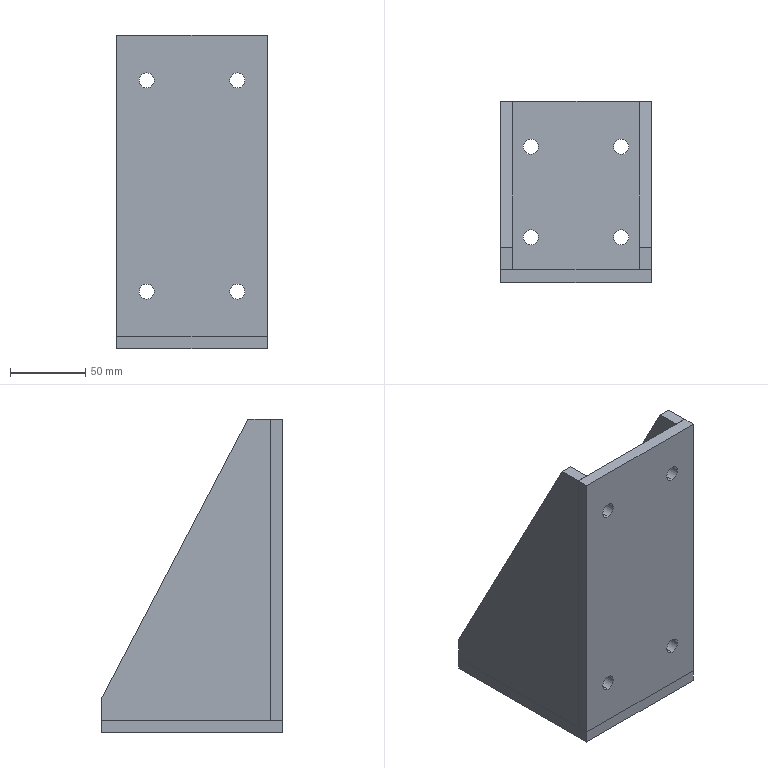Part | SolidWorks | features ICE 5, HoleWzd 3, Extrusion 1 | 4 solids | 42 faces | box 100 x 120 x 208 mm | volume 465813 mm3 | plane 26 | cylinder 16 | commonest cylinder face diameters 10 x16
STEP:
#1=CARTESIAN_POINT('',(-50.,-37.,208.));
#2=VERTEX_POINT('',#1);
#3=CARTESIAN_POINT('',(-50.,60.,23.));
#4=VERTEX_POINT('',#3);
#5=CARTESIAN_POINT('',(-50.,-37.,208.));
#6=DIRECTION('',(0.,0.4644,-0.8856));
#7=VECTOR('',#6,1000.);
#8=LINE('',#5,#7);
#9=EDGE_CURVE('',#2,#4,#8,.T.);
#10=ORIENTED_EDGE('',*,*,#9,.F.);
#11=CARTESIAN_POINT('',(-42.,-37.,208.));
#12=VERTEX_POINT('',#11);
#13=CARTESIAN_POINT('',(-42.,-37.,208.));
#14=DIRECTION('',(-1.,0.,0.));
#15=VECTOR('',#14,1000.);
#16=LINE('',#13,#15);
#17=EDGE_CURVE('',#12,#2,#16,.T.);
#18=ORIENTED_EDGE('',*,*,#17,.F.);
#19=CARTESIAN_POINT('',(-42.,60.,23.));
#20=VERTEX_POINT('',#19);
#21=CARTESIAN_POINT('',(-42.,-37.,208.));
#22=DIRECTION('',(0.,0.4644,-0.8856));
#23=VECTOR('',#22,1000.);
#24=LINE('',#21,#23);
#25=EDGE_CURVE('',#12,#20,#24,.T.);
#26=ORIENTED_EDGE('',*,*,#25,.T.);
#27=CARTESIAN_POINT('',(-42.,60.,23.));
#28=DIRECTION('',(-1.,0.,0.));
#29=VECTOR('',#28,1000.);
#30=LINE('',#27,#29);
#31=EDGE_CURVE('',#20,#4,#30,.T.);
#32=ORIENTED_EDGE('',*,*,#31,.T.);
#33=EDGE_LOOP('',(#10,#18,#26,#32));
#34=FACE_OUTER_BOUND('',#33,.T.);
#35=CARTESIAN_POINT('',(-42.,-37.,208.));
#36=DIRECTION('',(0.,0.8856,0.4644));
#37=DIRECTION('',(0.,-0.4644,0.8856));
#38=AXIS2_PLACEMENT_3D('',#35,#36,#37);
#39=PLANE('',#38);
#40=ADVANCED_FACE('',(#34),#39,.T.);
#41=CARTESIAN_POINT('',(-50.,-52.,208.));
#42=VERTEX_POINT('',#41);
#43=CARTESIAN_POINT('',(-50.,-52.,208.));
#44=DIRECTION('',(0.,1.,0.));
#45=VECTOR('',#44,1000.);
#46=LINE('',#43,#45);
#47=EDGE_CURVE('',#42,#2,#46,.T.);
#48=ORIENTED_EDGE('',*,*,#47,.F.);
#49=CARTESIAN_POINT('',(-42.,-52.,208.));
#50=VERTEX_POINT('',#49);
#51=CARTESIAN_POINT('',(-42.,-52.,208.));
#52=DIRECTION('',(-1.,0.,0.));
#53=VECTOR('',#52,1000.);
#54=LINE('',#51,#53);
#55=EDGE_CURVE('',#50,#42,#54,.T.);
#56=ORIENTED_EDGE('',*,*,#55,.F.);
#57=CARTESIAN_POINT('',(-42.,-52.,208.));
#58=DIRECTION('',(0.,1.,0.));
#59=VECTOR('',#58,1000.);
#60=LINE('',#57,#59);
#61=EDGE_CURVE('',#50,#12,#60,.T.);
#62=ORIENTED_EDGE('',*,*,#61,.T.);
#63=ORIENTED_EDGE('',*,*,#17,.T.);
#64=EDGE_LOOP('',(#48,#56,#62,#63));
#65=FACE_OUTER_BOUND('',#64,.T.);
#66=CARTESIAN_POINT('',(-42.,-52.,208.));
#67=DIRECTION('',(0.,0.,1.));
#68=DIRECTION('',(1.,0.,0.));
#69=AXIS2_PLACEMENT_3D('',#66,#67,#68);
#70=PLANE('',#69);
#71=ADVANCED_FACE('',(#65),#70,.T.);
#72=CARTESIAN_POINT('',(-50.,-52.,8.));
#73=VERTEX_POINT('',#72);
#74=CARTESIAN_POINT('',(-50.,-52.,8.));
#75=DIRECTION('',(0.,0.,1.));
#76=VECTOR('',#75,1000.);
#77=LINE('',#74,#76);
#78=EDGE_CURVE('',#73,#42,#77,.T.);
#79=ORIENTED_EDGE('',*,*,#78,.F.);
#80=CARTESIAN_POINT('',(-42.,-52.,8.));
#81=VERTEX_POINT('',#80);
#82=CARTESIAN_POINT('',(-42.,-52.,8.));
#83=DIRECTION('',(-1.,0.,0.));
#84=VECTOR('',#83,1000.);
#85=LINE('',#82,#84);
#86=EDGE_CURVE('',#81,#73,#85,.T.);
#87=ORIENTED_EDGE('',*,*,#86,.F.);
#88=CARTESIAN_POINT('',(-42.,-52.,8.));
#89=DIRECTION('',(0.,0.,1.));
#90=VECTOR('',#89,1000.);
#91=LINE('',#88,#90);
#92=EDGE_CURVE('',#81,#50,#91,.T.);
#93=ORIENTED_EDGE('',*,*,#92,.T.);
#94=ORIENTED_EDGE('',*,*,#55,.T.);
#95=EDGE_LOOP('',(#79,#87,#93,#94));
#96=FACE_OUTER_BOUND('',#95,.T.);
#97=CARTESIAN_POINT('',(-42.,-52.,8.));
#98=DIRECTION('',(0.,-1.,0.));
#99=DIRECTION('',(1.,0.,0.));
#100=AXIS2_PLACEMENT_3D('',#97,#98,#99);
#101=PLANE('',#100);
#102=ADVANCED_FACE('',(#96),#101,.T.);
#103=CARTESIAN_POINT('',(-50.,60.,8.));
#104=VERTEX_POINT('',#103);
#105=CARTESIAN_POINT('',(-50.,60.,8.));
#106=DIRECTION('',(0.,-1.,0.));
#107=VECTOR('',#106,1000.);
#108=LINE('',#105,#107);
#109=EDGE_CURVE('',#104,#73,#108,.T.);
#110=ORIENTED_EDGE('',*,*,#109,.F.);
#111=CARTESIAN_POINT('',(-42.,60.,8.));
#112=VERTEX_POINT('',#111);
#113=CARTESIAN_POINT('',(-42.,60.,8.));
#114=DIRECTION('',(-1.,0.,0.));
#115=VECTOR('',#114,1000.);
#116=LINE('',#113,#115);
#117=EDGE_CURVE('',#112,#104,#116,.T.);
#118=ORIENTED_EDGE('',*,*,#117,.F.);
#119=CARTESIAN_POINT('',(-42.,60.,8.));
#120=DIRECTION('',(0.,-1.,0.));
#121=VECTOR('',#120,1000.);
#122=LINE('',#119,#121);
#123=EDGE_CURVE('',#112,#81,#122,.T.);
#124=ORIENTED_EDGE('',*,*,#123,.T.);
#125=ORIENTED_EDGE('',*,*,#86,.T.);
#126=EDGE_LOOP('',(#110,#118,#124,#125));
#127=FACE_OUTER_BOUND('',#126,.T.);
#128=CARTESIAN_POINT('',(-42.,60.,8.));
#129=DIRECTION('',(0.,0.,-1.));
#130=DIRECTION('',(-1.,0.,0.));
#131=AXIS2_PLACEMENT_3D('',#128,#129,#130);
#132=PLANE('',#131);
#133=ADVANCED_FACE('',(#127),#132,.T.);
#134=CARTESIAN_POINT('',(-50.,60.,23.));
#135=DIRECTION('',(0.,0.,-1.));
#136=VECTOR('',#135,1000.);
#137=LINE('',#134,#136);
#138=EDGE_CURVE('',#4,#104,#137,.T.);
#139=ORIENTED_EDGE('',*,*,#138,.F.);
#140=ORIENTED_EDGE('',*,*,#31,.F.);
#141=CARTESIAN_POINT('',(-42.,60.,23.));
#142=DIRECTION('',(0.,0.,-1.));
#143=VECTOR('',#142,1000.);
#144=LINE('',#141,#143);
#145=EDGE_CURVE('',#20,#112,#144,.T.);
#146=ORIENTED_EDGE('',*,*,#145,.T.);
#147=ORIENTED_EDGE('',*,*,#117,.T.);
#148=EDGE_LOOP('',(#139,#140,#146,#147));
#149=FACE_OUTER_BOUND('',#148,.T.);
#150=CARTESIAN_POINT('',(-42.,60.,23.));
#151=DIRECTION('',(0.,1.,0.));
#152=DIRECTION('',(-1.,0.,0.));
#153=AXIS2_PLACEMENT_3D('',#150,#151,#152);
#154=PLANE('',#153);
#155=ADVANCED_FACE('',(#149),#154,.T.);
#156=ORIENTED_EDGE('',*,*,#25,.F.);
#157=ORIENTED_EDGE('',*,*,#61,.F.);
#158=ORIENTED_EDGE('',*,*,#92,.F.);
#159=ORIENTED_EDGE('',*,*,#123,.F.);
#160=ORIENTED_EDGE('',*,*,#145,.F.);
#161=EDGE_LOOP('',(#156,#157,#158,#159,#160));
#162=FACE_OUTER_BOUND('',#161,.T.);
#163=CARTESIAN_POINT('',(-42.,0.,0.));
#164=DIRECTION('',(-1.,0.,0.));
#165=DIRECTION('',(0.,-1.,0.));
#166=AXIS2_PLACEMENT_3D('',#163,#164,#165);
#167=PLANE('',#166);
#168=ADVANCED_FACE('',(#162),#167,.F.);
#169=ORIENTED_EDGE('',*,*,#9,.T.);
#170=ORIENTED_EDGE('',*,*,#138,.T.);
#171=ORIENTED_EDGE('',*,*,#109,.T.);
#172=ORIENTED_EDGE('',*,*,#78,.T.);
#173=ORIENTED_EDGE('',*,*,#47,.T.);
#174=EDGE_LOOP('',(#169,#170,#171,#172,#173));
#175=FACE_OUTER_BOUND('',#174,.T.);
#176=CARTESIAN_POINT('',(-50.,0.,0.));
#177=DIRECTION('',(-1.,0.,0.));
#178=DIRECTION('',(0.,-1.,0.));
#179=AXIS2_PLACEMENT_3D('',#176,#177,#178);
#180=PLANE('',#179);
#181=ADVANCED_FACE('',(#175),#180,.T.);
#182=CLOSED_SHELL('',(#40,#71,#102,#133,#155,#168,#181));
#183=MANIFOLD_SOLID_BREP('',#182);
#184=CARTESIAN_POINT('',(50.,-52.,208.));
#185=VERTEX_POINT('',#184);
#186=CARTESIAN_POINT('',(50.,-52.,8.));
#187=VERTEX_POINT('',#186);
#188=CARTESIAN_POINT('',(50.,-52.,208.));
#189=DIRECTION('',(0.,0.,-1.));
#190=VECTOR('',#189,1000.);
#191=LINE('',#188,#190);
#192=EDGE_CURVE('',#185,#187,#191,.T.);
#193=ORIENTED_EDGE('',*,*,#192,.F.);
#194=CARTESIAN_POINT('',(42.,-52.,208.));
#195=VERTEX_POINT('',#194);
#196=CARTESIAN_POINT('',(42.,-52.,208.));
#197=DIRECTION('',(1.,0.,0.));
#198=VECTOR('',#197,1000.);
#199=LINE('',#196,#198);
#200=EDGE_CURVE('',#195,#185,#199,.T.);
#201=ORIENTED_EDGE('',*,*,#200,.F.);
#202=CARTESIAN_POINT('',(42.,-52.,8.));
#203=VERTEX_POINT('',#202);
#204=CARTESIAN_POINT('',(42.,-52.,208.));
#205=DIRECTION('',(0.,0.,-1.));
#206=VECTOR('',#205,1000.);
#207=LINE('',#204,#206);
#208=EDGE_CURVE('',#195,#203,#207,.T.);
#209=ORIENTED_EDGE('',*,*,#208,.T.);
#210=CARTESIAN_POINT('',(42.,-52.,8.));
#211=DIRECTION('',(1.,0.,0.));
#212=VECTOR('',#211,1000.);
#213=LINE('',#210,#212);
#214=EDGE_CURVE('',#203,#187,#213,.T.);
#215=ORIENTED_EDGE('',*,*,#214,.T.);
#216=EDGE_LOOP('',(#193,#201,#209,#215));
#217=FACE_OUTER_BOUND('',#216,.T.);
#218=CARTESIAN_POINT('',(42.,-52.,208.));
#219=DIRECTION('',(0.,-1.,0.));
#220=DIRECTION('',(1.,0.,0.));
#221=AXIS2_PLACEMENT_3D('',#218,#219,#220);
#222=PLANE('',#221);
#223=ADVANCED_FACE('',(#217),#222,.T.);
#224=CARTESIAN_POINT('',(50.,-37.,208.));
#225=VERTEX_POINT('',#224);
#226=CARTESIAN_POINT('',(50.,-37.,208.));
#227=DIRECTION('',(0.,-1.,0.));
#228=VECTOR('',#227,1000.);
#229=LINE('',#226,#228);
#230=EDGE_CURVE('',#225,#185,#229,.T.);
#231=ORIENTED_EDGE('',*,*,#230,.F.);
#232=CARTESIAN_POINT('',(42.,-37.,208.));
#233=VERTEX_POINT('',#232);
#234=CARTESIAN_POINT('',(42.,-37.,208.));
#235=DIRECTION('',(1.,0.,0.));
#236=VECTOR('',#235,1000.);
#237=LINE('',#234,#236);
#238=EDGE_CURVE('',#233,#225,#237,.T.);
#239=ORIENTED_EDGE('',*,*,#238,.F.);
#240=CARTESIAN_POINT('',(42.,-37.,208.));
#241=DIRECTION('',(0.,-1.,0.));
#242=VECTOR('',#241,1000.);
#243=LINE('',#240,#242);
#244=EDGE_CURVE('',#233,#195,#243,.T.);
#245=ORIENTED_EDGE('',*,*,#244,.T.);
#246=ORIENTED_EDGE('',*,*,#200,.T.);
#247=EDGE_LOOP('',(#231,#239,#245,#246));
#248=FACE_OUTER_BOUND('',#247,.T.);
#249=CARTESIAN_POINT('',(42.,-37.,208.));
#250=DIRECTION('',(0.,0.,1.));
#251=DIRECTION('',(1.,0.,0.));
#252=AXIS2_PLACEMENT_3D('',#249,#250,#251);
#253=PLANE('',#252);
#254=ADVANCED_FACE('',(#248),#253,.T.);
#255=CARTESIAN_POINT('',(50.,60.,23.));
#256=VERTEX_POINT('',#255);
#257=CARTESIAN_POINT('',(50.,60.,23.));
#258=DIRECTION('',(0.,-0.4644,0.8856));
#259=VECTOR('',#258,1000.);
#260=LINE('',#257,#259);
#261=EDGE_CURVE('',#256,#225,#260,.T.);
#262=ORIENTED_EDGE('',*,*,#261,.F.);
#263=CARTESIAN_POINT('',(42.,60.,23.));
#264=VERTEX_POINT('',#263);
#265=CARTESIAN_POINT('',(42.,60.,23.));
#266=DIRECTION('',(1.,0.,0.));
#267=VECTOR('',#266,1000.);
#268=LINE('',#265,#267);
#269=EDGE_CURVE('',#264,#256,#268,.T.);
#270=ORIENTED_EDGE('',*,*,#269,.F.);
#271=CARTESIAN_POINT('',(42.,60.,23.));
#272=DIRECTION('',(0.,-0.4644,0.8856));
#273=VECTOR('',#272,1000.);
#274=LINE('',#271,#273);
#275=EDGE_CURVE('',#264,#233,#274,.T.);
#276=ORIENTED_EDGE('',*,*,#275,.T.);
#277=ORIENTED_EDGE('',*,*,#238,.T.);
#278=EDGE_LOOP('',(#262,#270,#276,#277));
#279=FACE_OUTER_BOUND('',#278,.T.);
#280=CARTESIAN_POINT('',(42.,60.,23.));
#281=DIRECTION('',(0.,0.8856,0.4644));
#282=DIRECTION('',(0.,-0.4644,0.8856));
#283=AXIS2_PLACEMENT_3D('',#280,#281,#282);
#284=PLANE('',#283);
#285=ADVANCED_FACE('',(#279),#284,.T.);
#286=CARTESIAN_POINT('',(50.,60.,8.));
#287=VERTEX_POINT('',#286);
#288=CARTESIAN_POINT('',(50.,60.,8.));
#289=DIRECTION('',(0.,0.,1.));
#290=VECTOR('',#289,1000.);
#291=LINE('',#288,#290);
#292=EDGE_CURVE('',#287,#256,#291,.T.);
#293=ORIENTED_EDGE('',*,*,#292,.F.);
#294=CARTESIAN_POINT('',(42.,60.,8.));
#295=VERTEX_POINT('',#294);
#296=CARTESIAN_POINT('',(42.,60.,8.));
#297=DIRECTION('',(1.,0.,0.));
#298=VECTOR('',#297,1000.);
#299=LINE('',#296,#298);
#300=EDGE_CURVE('',#295,#287,#299,.T.);
#301=ORIENTED_EDGE('',*,*,#300,.F.);
#302=CARTESIAN_POINT('',(42.,60.,8.));
#303=DIRECTION('',(0.,0.,1.));
#304=VECTOR('',#303,1000.);
#305=LINE('',#302,#304);
#306=EDGE_CURVE('',#295,#264,#305,.T.);
#307=ORIENTED_EDGE('',*,*,#306,.T.);
#308=ORIENTED_EDGE('',*,*,#269,.T.);
#309=EDGE_LOOP('',(#293,#301,#307,#308));
#310=FACE_OUTER_BOUND('',#309,.T.);
#311=CARTESIAN_POINT('',(42.,60.,8.));
#312=DIRECTION('',(0.,1.,0.));
#313=DIRECTION('',(-1.,0.,0.));
#314=AXIS2_PLACEMENT_3D('',#311,#312,#313);
#315=PLANE('',#314);
#316=ADVANCED_FACE('',(#310),#315,.T.);
#317=CARTESIAN_POINT('',(50.,-52.,8.));
#318=DIRECTION('',(0.,1.,0.));
#319=VECTOR('',#318,1000.);
#320=LINE('',#317,#319);
#321=EDGE_CURVE('',#187,#287,#320,.T.);
#322=ORIENTED_EDGE('',*,*,#321,.F.);
#323=ORIENTED_EDGE('',*,*,#214,.F.);
#324=CARTESIAN_POINT('',(42.,-52.,8.));
#325=DIRECTION('',(0.,1.,0.));
#326=VECTOR('',#325,1000.);
#327=LINE('',#324,#326);
#328=EDGE_CURVE('',#203,#295,#327,.T.);
#329=ORIENTED_EDGE('',*,*,#328,.T.);
#330=ORIENTED_EDGE('',*,*,#300,.T.);
#331=EDGE_LOOP('',(#322,#323,#329,#330));
#332=FACE_OUTER_BOUND('',#331,.T.);
#333=CARTESIAN_POINT('',(42.,-52.,8.));
#334=DIRECTION('',(0.,0.,-1.));
#335=DIRECTION('',(-1.,0.,0.));
#336=AXIS2_PLACEMENT_3D('',#333,#334,#335);
#337=PLANE('',#336);
#338=ADVANCED_FACE('',(#332),#337,.T.);
#339=ORIENTED_EDGE('',*,*,#208,.F.);
#340=ORIENTED_EDGE('',*,*,#244,.F.);
#341=ORIENTED_EDGE('',*,*,#275,.F.);
#342=ORIENTED_EDGE('',*,*,#306,.F.);
#343=ORIENTED_EDGE('',*,*,#328,.F.);
#344=EDGE_LOOP('',(#339,#340,#341,#342,#343));
#345=FACE_OUTER_BOUND('',#344,.T.);
#346=CARTESIAN_POINT('',(42.,0.,0.));
#347=DIRECTION('',(1.,0.,0.));
#348=DIRECTION('',(0.,1.,0.));
#349=AXIS2_PLACEMENT_3D('',#346,#347,#348);
#350=PLANE('',#349);
#351=ADVANCED_FACE('',(#345),#350,.F.);
#352=ORIENTED_EDGE('',*,*,#192,.T.);
#353=ORIENTED_EDGE('',*,*,#321,.T.);
#354=ORIENTED_EDGE('',*,*,#292,.T.);
#355=ORIENTED_EDGE('',*,*,#261,.T.);
#356=ORIENTED_EDGE('',*,*,#230,.T.);
#357=EDGE_LOOP('',(#352,#353,#354,#355,#356));
#358=FACE_OUTER_BOUND('',#357,.T.);
#359=CARTESIAN_POINT('',(50.,0.,0.));
#360=DIRECTION('',(1.,0.,0.));
#361=DIRECTION('',(0.,1.,0.));
#362=AXIS2_PLACEMENT_3D('',#359,#360,#361);
#363=PLANE('',#362);
#364=ADVANCED_FACE('',(#358),#363,.T.);
#365=CLOSED_SHELL('',(#223,#254,#285,#316,#338,#351,#364));
#366=MANIFOLD_SOLID_BREP('',#365);
#367=CARTESIAN_POINT('',(-30.,-60.,33.));
#368=VERTEX_POINT('',#367);
#369=CARTESIAN_POINT('',(-30.,-60.,43.));
#370=VERTEX_POINT('',#369);
#371=CARTESIAN_POINT('',(-30.,-60.,38.));
#372=DIRECTION('',(0.,1.,0.));
#373=DIRECTION('',(0.,0.,1.));
#374=AXIS2_PLACEMENT_3D('',#371,#372,#373);
#375=CIRCLE('',#374,5.);
#376=EDGE_CURVE('',#368,#370,#375,.T.);
#377=ORIENTED_EDGE('',*,*,#376,.F.);
#378=CARTESIAN_POINT('',(-30.,-52.,33.));
#379=VERTEX_POINT('',#378);
#380=CARTESIAN_POINT('',(-30.,-52.,33.));
#381=DIRECTION('',(0.,1.,0.));
#382=VECTOR('',#381,1000.);
#383=LINE('',#380,#382);
#384=EDGE_CURVE('',#368,#379,#383,.T.);
#385=ORIENTED_EDGE('',*,*,#384,.T.);
#386=CARTESIAN_POINT('',(-30.,-52.,43.));
#387=VERTEX_POINT('',#386);
#388=CARTESIAN_POINT('',(-30.,-52.,38.));
#389=DIRECTION('',(0.,1.,0.));
#390=DIRECTION('',(0.,0.,1.));
#391=AXIS2_PLACEMENT_3D('',#388,#389,#390);
#392=CIRCLE('',#391,5.);
#393=EDGE_CURVE('',#379,#387,#392,.T.);
#394=ORIENTED_EDGE('',*,*,#393,.T.);
#395=CARTESIAN_POINT('',(-30.,-52.,43.));
#396=DIRECTION('',(0.,1.,0.));
#397=VECTOR('',#396,1000.);
#398=LINE('',#395,#397);
#399=EDGE_CURVE('',#370,#387,#398,.T.);
#400=ORIENTED_EDGE('',*,*,#399,.F.);
#401=EDGE_LOOP('',(#377,#385,#394,#400));
#402=FACE_OUTER_BOUND('',#401,.T.);
#403=CARTESIAN_POINT('',(-30.,-52.,38.));
#404=DIRECTION('',(0.,1.,0.));
#405=DIRECTION('',(0.,0.,1.));
#406=AXIS2_PLACEMENT_3D('',#403,#404,#405);
#407=CYLINDRICAL_SURFACE('',#406,5.);
#408=ADVANCED_FACE('',(#402),#407,.F.);
#409=CARTESIAN_POINT('',(30.,-60.,33.));
#410=VERTEX_POINT('',#409);
#411=CARTESIAN_POINT('',(30.,-60.,43.));
#412=VERTEX_POINT('',#411);
#413=CARTESIAN_POINT('',(30.,-60.,38.));
#414=DIRECTION('',(0.,1.,0.));
#415=DIRECTION('',(0.,0.,1.));
#416=AXIS2_PLACEMENT_3D('',#413,#414,#415);
#417=CIRCLE('',#416,5.);
#418=EDGE_CURVE('',#410,#412,#417,.T.);
#419=ORIENTED_EDGE('',*,*,#418,.F.);
#420=CARTESIAN_POINT('',(30.,-52.,33.));
#421=VERTEX_POINT('',#420);
#422=CARTESIAN_POINT('',(30.,-52.,33.));
#423=DIRECTION('',(0.,1.,0.));
#424=VECTOR('',#423,1000.);
#425=LINE('',#422,#424);
#426=EDGE_CURVE('',#410,#421,#425,.T.);
#427=ORIENTED_EDGE('',*,*,#426,.T.);
#428=CARTESIAN_POINT('',(30.,-52.,43.));
#429=VERTEX_POINT('',#428);
#430=CARTESIAN_POINT('',(30.,-52.,38.));
#431=DIRECTION('',(0.,1.,0.));
#432=DIRECTION('',(0.,0.,1.));
#433=AXIS2_PLACEMENT_3D('',#430,#431,#432);
#434=CIRCLE('',#433,5.);
#435=EDGE_CURVE('',#421,#429,#434,.T.);
#436=ORIENTED_EDGE('',*,*,#435,.T.);
#437=CARTESIAN_POINT('',(30.,-52.,43.));
#438=DIRECTION('',(0.,1.,0.));
#439=VECTOR('',#438,1000.);
#440=LINE('',#437,#439);
#441=EDGE_CURVE('',#412,#429,#440,.T.);
#442=ORIENTED_EDGE('',*,*,#441,.F.);
#443=EDGE_LOOP('',(#419,#427,#436,#442));
#444=FACE_OUTER_BOUND('',#443,.T.);
#445=CARTESIAN_POINT('',(30.,-52.,38.));
#446=DIRECTION('',(0.,1.,0.));
#447=DIRECTION('',(0.,0.,1.));
#448=AXIS2_PLACEMENT_3D('',#445,#446,#447);
#449=CYLINDRICAL_SURFACE('',#448,5.);
#450=ADVANCED_FACE('',(#444),#449,.F.);
#451=CARTESIAN_POINT('',(-30.,-60.,173.));
#452=VERTEX_POINT('',#451);
#453=CARTESIAN_POINT('',(-30.,-60.,183.));
#454=VERTEX_POINT('',#453);
#455=CARTESIAN_POINT('',(-30.,-60.,178.));
#456=DIRECTION('',(0.,1.,0.));
#457=DIRECTION('',(0.,0.,1.));
#458=AXIS2_PLACEMENT_3D('',#455,#456,#457);
#459=CIRCLE('',#458,5.);
#460=EDGE_CURVE('',#452,#454,#459,.T.);
#461=ORIENTED_EDGE('',*,*,#460,.F.);
#462=CARTESIAN_POINT('',(-30.,-52.,173.));
#463=VERTEX_POINT('',#462);
#464=CARTESIAN_POINT('',(-30.,-52.,173.));
#465=DIRECTION('',(0.,1.,0.));
#466=VECTOR('',#465,1000.);
#467=LINE('',#464,#466);
#468=EDGE_CURVE('',#452,#463,#467,.T.);
#469=ORIENTED_EDGE('',*,*,#468,.T.);
#470=CARTESIAN_POINT('',(-30.,-52.,183.));
#471=VERTEX_POINT('',#470);
#472=CARTESIAN_POINT('',(-30.,-52.,178.));
#473=DIRECTION('',(0.,1.,0.));
#474=DIRECTION('',(0.,0.,1.));
#475=AXIS2_PLACEMENT_3D('',#472,#473,#474);
#476=CIRCLE('',#475,5.);
#477=EDGE_CURVE('',#463,#471,#476,.T.);
#478=ORIENTED_EDGE('',*,*,#477,.T.);
#479=CARTESIAN_POINT('',(-30.,-52.,183.));
#480=DIRECTION('',(0.,1.,0.));
#481=VECTOR('',#480,1000.);
#482=LINE('',#479,#481);
#483=EDGE_CURVE('',#454,#471,#482,.T.);
#484=ORIENTED_EDGE('',*,*,#483,.F.);
#485=EDGE_LOOP('',(#461,#469,#478,#484));
#486=FACE_OUTER_BOUND('',#485,.T.);
#487=CARTESIAN_POINT('',(-30.,-52.,178.));
#488=DIRECTION('',(0.,1.,0.));
#489=DIRECTION('',(0.,0.,1.));
#490=AXIS2_PLACEMENT_3D('',#487,#488,#489);
#491=CYLINDRICAL_SURFACE('',#490,5.);
#492=ADVANCED_FACE('',(#486),#491,.F.);
#493=CARTESIAN_POINT('',(30.,-60.,173.));
#494=VERTEX_POINT('',#493);
#495=CARTESIAN_POINT('',(30.,-60.,183.));
#496=VERTEX_POINT('',#495);
#497=CARTESIAN_POINT('',(30.,-60.,178.));
#498=DIRECTION('',(0.,1.,0.));
#499=DIRECTION('',(0.,0.,1.));
#500=AXIS2_PLACEMENT_3D('',#497,#498,#499);
#501=CIRCLE('',#500,5.);
#502=EDGE_CURVE('',#494,#496,#501,.T.);
#503=ORIENTED_EDGE('',*,*,#502,.F.);
#504=CARTESIAN_POINT('',(30.,-52.,173.));
#505=VERTEX_POINT('',#504);
#506=CARTESIAN_POINT('',(30.,-52.,173.));
#507=DIRECTION('',(0.,1.,0.));
#508=VECTOR('',#507,1000.);
#509=LINE('',#506,#508);
#510=EDGE_CURVE('',#494,#505,#509,.T.);
#511=ORIENTED_EDGE('',*,*,#510,.T.);
#512=CARTESIAN_POINT('',(30.,-52.,183.));
#513=VERTEX_POINT('',#512);
#514=CARTESIAN_POINT('',(30.,-52.,178.));
#515=DIRECTION('',(0.,1.,0.));
#516=DIRECTION('',(0.,0.,1.));
#517=AXIS2_PLACEMENT_3D('',#514,#515,#516);
#518=CIRCLE('',#517,5.);
#519=EDGE_CURVE('',#505,#513,#518,.T.);
#520=ORIENTED_EDGE('',*,*,#519,.T.);
#521=CARTESIAN_POINT('',(30.,-52.,183.));
#522=DIRECTION('',(0.,1.,0.));
#523=VECTOR('',#522,1000.);
#524=LINE('',#521,#523);
#525=EDGE_CURVE('',#496,#513,#524,.T.);
#526=ORIENTED_EDGE('',*,*,#525,.F.);
#527=EDGE_LOOP('',(#503,#511,#520,#526));
#528=FACE_OUTER_BOUND('',#527,.T.);
#529=CARTESIAN_POINT('',(30.,-52.,178.));
#530=DIRECTION('',(0.,1.,0.));
#531=DIRECTION('',(0.,0.,1.));
#532=AXIS2_PLACEMENT_3D('',#529,#530,#531);
#533=CYLINDRICAL_SURFACE('',#532,5.);
#534=ADVANCED_FACE('',(#528),#533,.F.);
#535=CARTESIAN_POINT('',(-50.,-52.,8.));
#536=VERTEX_POINT('',#535);
#537=CARTESIAN_POINT('',(-50.,-60.,8.));
#538=VERTEX_POINT('',#537);
#539=CARTESIAN_POINT('',(-50.,-60.,8.));
#540=DIRECTION('',(0.,-1.,0.));
#541=VECTOR('',#540,1000.);
#542=LINE('',#539,#541);
#543=EDGE_CURVE('',#536,#538,#542,.T.);
#544=ORIENTED_EDGE('',*,*,#543,.T.);
#545=CARTESIAN_POINT('',(-50.,-60.,208.));
#546=VERTEX_POINT('',#545);
#547=CARTESIAN_POINT('',(-50.,-60.,208.));
#548=DIRECTION('',(0.,0.,-1.));
#549=VECTOR('',#548,1000.);
#550=LINE('',#547,#549);
#551=EDGE_CURVE('',#546,#538,#550,.T.);
#552=ORIENTED_EDGE('',*,*,#551,.F.);
#553=CARTESIAN_POINT('',(-50.,-52.,208.));
#554=VERTEX_POINT('',#553);
#555=CARTESIAN_POINT('',(-50.,-60.,208.));
#556=DIRECTION('',(0.,-1.,0.));
#557=VECTOR('',#556,1000.);
#558=LINE('',#555,#557);
#559=EDGE_CURVE('',#554,#546,#558,.T.);
#560=ORIENTED_EDGE('',*,*,#559,.F.);
#561=CARTESIAN_POINT('',(-50.,-52.,208.));
#562=DIRECTION('',(0.,0.,-1.));
#563=VECTOR('',#562,1000.);
#564=LINE('',#561,#563);
#565=EDGE_CURVE('',#554,#536,#564,.T.);
#566=ORIENTED_EDGE('',*,*,#565,.T.);
#567=EDGE_LOOP('',(#544,#552,#560,#566));
#568=FACE_OUTER_BOUND('',#567,.T.);
#569=CARTESIAN_POINT('',(-50.,-60.,208.));
#570=DIRECTION('',(1.,0.,0.));
#571=DIRECTION('',(0.,0.,-1.));
#572=AXIS2_PLACEMENT_3D('',#569,#570,#571);
#573=PLANE('',#572);
#574=ADVANCED_FACE('',(#568),#573,.F.);
#575=CARTESIAN_POINT('',(-30.,-60.,38.));
#576=DIRECTION('',(0.,1.,0.));
#577=DIRECTION('',(0.,0.,1.));
#578=AXIS2_PLACEMENT_3D('',#575,#576,#577);
#579=CIRCLE('',#578,5.);
#580=EDGE_CURVE('',#370,#368,#579,.T.);
#581=ORIENTED_EDGE('',*,*,#580,.T.);
#582=ORIENTED_EDGE('',*,*,#376,.T.);
#583=EDGE_LOOP('',(#581,#582));
#584=FACE_BOUND('',#583,.T.);
#585=CARTESIAN_POINT('',(30.,-60.,38.));
#586=DIRECTION('',(0.,1.,0.));
#587=DIRECTION('',(0.,0.,1.));
#588=AXIS2_PLACEMENT_3D('',#585,#586,#587);
#589=CIRCLE('',#588,5.);
#590=EDGE_CURVE('',#412,#410,#589,.T.);
#591=ORIENTED_EDGE('',*,*,#590,.T.);
#592=ORIENTED_EDGE('',*,*,#418,.T.);
#593=EDGE_LOOP('',(#591,#592));
#594=FACE_BOUND('',#593,.T.);
#595=CARTESIAN_POINT('',(-30.,-60.,178.));
#596=DIRECTION('',(0.,1.,0.));
#597=DIRECTION('',(0.,0.,1.));
#598=AXIS2_PLACEMENT_3D('',#595,#596,#597);
#599=CIRCLE('',#598,5.);
#600=EDGE_CURVE('',#454,#452,#599,.T.);
#601=ORIENTED_EDGE('',*,*,#600,.T.);
#602=ORIENTED_EDGE('',*,*,#460,.T.);
#603=EDGE_LOOP('',(#601,#602));
#604=FACE_BOUND('',#603,.T.);
#605=CARTESIAN_POINT('',(30.,-60.,178.));
#606=DIRECTION('',(0.,1.,0.));
#607=DIRECTION('',(0.,0.,1.));
#608=AXIS2_PLACEMENT_3D('',#605,#606,#607);
#609=CIRCLE('',#608,5.);
#610=EDGE_CURVE('',#496,#494,#609,.T.);
#611=ORIENTED_EDGE('',*,*,#610,.T.);
#612=ORIENTED_EDGE('',*,*,#502,.T.);
#613=EDGE_LOOP('',(#611,#612));
#614=FACE_BOUND('',#613,.T.);
#615=CARTESIAN_POINT('',(50.,-60.,8.));
#616=VERTEX_POINT('',#615);
#617=CARTESIAN_POINT('',(-50.,-60.,8.));
#618=DIRECTION('',(1.,0.,0.));
#619=VECTOR('',#618,1000.);
#620=LINE('',#617,#619);
#621=EDGE_CURVE('',#538,#616,#620,.T.);
#622=ORIENTED_EDGE('',*,*,#621,.T.);
#623=CARTESIAN_POINT('',(50.,-60.,208.));
#624=VERTEX_POINT('',#623);
#625=CARTESIAN_POINT('',(50.,-60.,208.));
#626=DIRECTION('',(0.,0.,-1.));
#627=VECTOR('',#626,1000.);
#628=LINE('',#625,#627);
#629=EDGE_CURVE('',#624,#616,#628,.T.);
#630=ORIENTED_EDGE('',*,*,#629,.F.);
#631=CARTESIAN_POINT('',(-50.,-60.,208.));
#632=DIRECTION('',(1.,0.,0.));
#633=VECTOR('',#632,1000.);
#634=LINE('',#631,#633);
#635=EDGE_CURVE('',#546,#624,#634,.T.);
#636=ORIENTED_EDGE('',*,*,#635,.F.);
#637=ORIENTED_EDGE('',*,*,#551,.T.);
#638=EDGE_LOOP('',(#622,#630,#636,#637));
#639=FACE_OUTER_BOUND('',#638,.T.);
#640=CARTESIAN_POINT('',(-50.,-60.,208.));
#641=DIRECTION('',(0.,1.,0.));
#642=DIRECTION('',(0.,0.,1.));
#643=AXIS2_PLACEMENT_3D('',#640,#641,#642);
#644=PLANE('',#643);
#645=ADVANCED_FACE('',(#584,#594,#604,#614,#639),#644,.F.);
#646=CARTESIAN_POINT('',(50.,-52.,8.));
#647=VERTEX_POINT('',#646);
#648=CARTESIAN_POINT('',(50.,-60.,8.));
#649=DIRECTION('',(0.,1.,0.));
#650=VECTOR('',#649,1000.);
#651=LINE('',#648,#650);
#652=EDGE_CURVE('',#616,#647,#651,.T.);
#653=ORIENTED_EDGE('',*,*,#652,.T.);
#654=CARTESIAN_POINT('',(50.,-52.,208.));
#655=VERTEX_POINT('',#654);
#656=CARTESIAN_POINT('',(50.,-52.,208.));
#657=DIRECTION('',(0.,0.,-1.));
#658=VECTOR('',#657,1000.);
#659=LINE('',#656,#658);
#660=EDGE_CURVE('',#655,#647,#659,.T.);
#661=ORIENTED_EDGE('',*,*,#660,.F.);
#662=CARTESIAN_POINT('',(50.,-60.,208.));
#663=DIRECTION('',(0.,1.,0.));
#664=VECTOR('',#663,1000.);
#665=LINE('',#662,#664);
#666=EDGE_CURVE('',#624,#655,#665,.T.);
#667=ORIENTED_EDGE('',*,*,#666,.F.);
#668=ORIENTED_EDGE('',*,*,#629,.T.);
#669=EDGE_LOOP('',(#653,#661,#667,#668));
#670=FACE_OUTER_BOUND('',#669,.T.);
#671=CARTESIAN_POINT('',(50.,-60.,208.));
#672=DIRECTION('',(-1.,0.,0.));
#673=DIRECTION('',(0.,0.,1.));
#674=AXIS2_PLACEMENT_3D('',#671,#672,#673);
#675=PLANE('',#674);
#676=ADVANCED_FACE('',(#670),#675,.F.);
#677=CARTESIAN_POINT('',(-30.,-52.,38.));
#678=DIRECTION('',(0.,1.,0.));
#679=DIRECTION('',(0.,0.,1.));
#680=AXIS2_PLACEMENT_3D('',#677,#678,#679);
#681=CIRCLE('',#680,5.);
#682=EDGE_CURVE('',#387,#379,#681,.T.);
#683=ORIENTED_EDGE('',*,*,#682,.F.);
#684=ORIENTED_EDGE('',*,*,#393,.F.);
#685=EDGE_LOOP('',(#683,#684));
#686=FACE_BOUND('',#685,.T.);
#687=CARTESIAN_POINT('',(30.,-52.,38.));
#688=DIRECTION('',(0.,1.,0.));
#689=DIRECTION('',(0.,0.,1.));
#690=AXIS2_PLACEMENT_3D('',#687,#688,#689);
#691=CIRCLE('',#690,5.);
#692=EDGE_CURVE('',#429,#421,#691,.T.);
#693=ORIENTED_EDGE('',*,*,#692,.F.);
#694=ORIENTED_EDGE('',*,*,#435,.F.);
#695=EDGE_LOOP('',(#693,#694));
#696=FACE_BOUND('',#695,.T.);
#697=CARTESIAN_POINT('',(-30.,-52.,178.));
#698=DIRECTION('',(0.,1.,0.));
#699=DIRECTION('',(0.,0.,1.));
#700=AXIS2_PLACEMENT_3D('',#697,#698,#699);
#701=CIRCLE('',#700,5.);
#702=EDGE_CURVE('',#471,#463,#701,.T.);
#703=ORIENTED_EDGE('',*,*,#702,.F.);
#704=ORIENTED_EDGE('',*,*,#477,.F.);
#705=EDGE_LOOP('',(#703,#704));
#706=FACE_BOUND('',#705,.T.);
#707=CARTESIAN_POINT('',(30.,-52.,178.));
#708=DIRECTION('',(0.,1.,0.));
#709=DIRECTION('',(0.,0.,1.));
#710=AXIS2_PLACEMENT_3D('',#707,#708,#709);
#711=CIRCLE('',#710,5.);
#712=EDGE_CURVE('',#513,#505,#711,.T.);
#713=ORIENTED_EDGE('',*,*,#712,.F.);
#714=ORIENTED_EDGE('',*,*,#519,.F.);
#715=EDGE_LOOP('',(#713,#714));
#716=FACE_BOUND('',#715,.T.);
#717=CARTESIAN_POINT('',(-50.,-52.,8.));
#718=DIRECTION('',(-1.,0.,0.));
#719=VECTOR('',#718,1000.);
#720=LINE('',#717,#719);
#721=EDGE_CURVE('',#647,#536,#720,.T.);
#722=ORIENTED_EDGE('',*,*,#721,.T.);
#723=ORIENTED_EDGE('',*,*,#565,.F.);
#724=CARTESIAN_POINT('',(-50.,-52.,208.));
#725=DIRECTION('',(-1.,0.,0.));
#726=VECTOR('',#725,1000.);
#727=LINE('',#724,#726);
#728=EDGE_CURVE('',#655,#554,#727,.T.);
#729=ORIENTED_EDGE('',*,*,#728,.F.);
#730=ORIENTED_EDGE('',*,*,#660,.T.);
#731=EDGE_LOOP('',(#722,#723,#729,#730));
#732=FACE_OUTER_BOUND('',#731,.T.);
#733=CARTESIAN_POINT('',(-50.,-52.,208.));
#734=DIRECTION('',(0.,-1.,0.));
#735=DIRECTION('',(0.,0.,-1.));
#736=AXIS2_PLACEMENT_3D('',#733,#734,#735);
#737=PLANE('',#736);
#738=ADVANCED_FACE('',(#686,#696,#706,#716,#732),#737,.F.);
#739=ORIENTED_EDGE('',*,*,#559,.T.);
#740=ORIENTED_EDGE('',*,*,#635,.T.);
#741=ORIENTED_EDGE('',*,*,#666,.T.);
#742=ORIENTED_EDGE('',*,*,#728,.T.);
#743=EDGE_LOOP('',(#739,#740,#741,#742));
#744=FACE_OUTER_BOUND('',#743,.T.);
#745=CARTESIAN_POINT('',(0.,0.,208.));
#746=DIRECTION('',(0.,0.,-1.));
#747=DIRECTION('',(-1.,0.,0.));
#748=AXIS2_PLACEMENT_3D('',#745,#746,#747);
#749=PLANE('',#748);
#750=ADVANCED_FACE('',(#744),#749,.F.);
#751=ORIENTED_EDGE('',*,*,#543,.F.);
#752=ORIENTED_EDGE('',*,*,#721,.F.);
#753=ORIENTED_EDGE('',*,*,#652,.F.);
#754=ORIENTED_EDGE('',*,*,#621,.F.);
#755=EDGE_LOOP('',(#751,#752,#753,#754));
#756=FACE_OUTER_BOUND('',#755,.T.);
#757=CARTESIAN_POINT('',(0.,0.,8.));
#758=DIRECTION('',(0.,0.,-1.));
#759=DIRECTION('',(-1.,0.,0.));
#760=AXIS2_PLACEMENT_3D('',#757,#758,#759);
#761=PLANE('',#760);
#762=ADVANCED_FACE('',(#756),#761,.T.);
#763=ORIENTED_EDGE('',*,*,#510,.F.);
#764=ORIENTED_EDGE('',*,*,#610,.F.);
#765=ORIENTED_EDGE('',*,*,#525,.T.);
#766=ORIENTED_EDGE('',*,*,#712,.T.);
#767=EDGE_LOOP('',(#763,#764,#765,#766));
#768=FACE_OUTER_BOUND('',#767,.T.);
#769=CARTESIAN_POINT('',(30.,-52.,178.));
#770=DIRECTION('',(0.,1.,0.));
#771=DIRECTION('',(0.,0.,1.));
#772=AXIS2_PLACEMENT_3D('',#769,#770,#771);
#773=CYLINDRICAL_SURFACE('',#772,5.);
#774=ADVANCED_FACE('',(#768),#773,.F.);
#775=ORIENTED_EDGE('',*,*,#468,.F.);
#776=ORIENTED_EDGE('',*,*,#600,.F.);
#777=ORIENTED_EDGE('',*,*,#483,.T.);
#778=ORIENTED_EDGE('',*,*,#702,.T.);
#779=EDGE_LOOP('',(#775,#776,#777,#778));
#780=FACE_OUTER_BOUND('',#779,.T.);
#781=CARTESIAN_POINT('',(-30.,-52.,178.));
#782=DIRECTION('',(0.,1.,0.));
#783=DIRECTION('',(0.,0.,1.));
#784=AXIS2_PLACEMENT_3D('',#781,#782,#783);
#785=CYLINDRICAL_SURFACE('',#784,5.);
#786=ADVANCED_FACE('',(#780),#785,.F.);
#787=ORIENTED_EDGE('',*,*,#426,.F.);
#788=ORIENTED_EDGE('',*,*,#590,.F.);
#789=ORIENTED_EDGE('',*,*,#441,.T.);
#790=ORIENTED_EDGE('',*,*,#692,.T.);
#791=EDGE_LOOP('',(#787,#788,#789,#790));
#792=FACE_OUTER_BOUND('',#791,.T.);
#793=CARTESIAN_POINT('',(30.,-52.,38.));
#794=DIRECTION('',(0.,1.,0.));
#795=DIRECTION('',(0.,0.,1.));
#796=AXIS2_PLACEMENT_3D('',#793,#794,#795);
#797=CYLINDRICAL_SURFACE('',#796,5.);
#798=ADVANCED_FACE('',(#792),#797,.F.);
#799=ORIENTED_EDGE('',*,*,#384,.F.);
#800=ORIENTED_EDGE('',*,*,#580,.F.);
#801=ORIENTED_EDGE('',*,*,#399,.T.);
#802=ORIENTED_EDGE('',*,*,#682,.T.);
#803=EDGE_LOOP('',(#799,#800,#801,#802));
#804=FACE_OUTER_BOUND('',#803,.T.);
#805=CARTESIAN_POINT('',(-30.,-52.,38.));
#806=DIRECTION('',(0.,1.,0.));
#807=DIRECTION('',(0.,0.,1.));
#808=AXIS2_PLACEMENT_3D('',#805,#806,#807);
#809=CYLINDRICAL_SURFACE('',#808,5.);
#810=ADVANCED_FACE('',(#804),#809,.F.);
#811=CLOSED_SHELL('',(#408,#450,#492,#534,#574,#645,#676,#738,#750,#762,#774,#786,#798,#810));
#812=MANIFOLD_SOLID_BREP('',#811);
#813=CARTESIAN_POINT('',(25.,30.,8.));
#814=VERTEX_POINT('',#813);
#815=CARTESIAN_POINT('',(35.,30.,8.));
#816=VERTEX_POINT('',#815);
#817=CARTESIAN_POINT('',(30.,30.,8.));
#818=DIRECTION('',(0.,0.,1.));
#819=DIRECTION('',(1.,0.,0.));
#820=AXIS2_PLACEMENT_3D('',#817,#818,#819);
#821=CIRCLE('',#820,5.);
#822=EDGE_CURVE('',#814,#816,#821,.T.);
#823=ORIENTED_EDGE('',*,*,#822,.T.);
#824=CARTESIAN_POINT('',(35.,30.,0.));
#825=VERTEX_POINT('',#824);
#826=CARTESIAN_POINT('',(35.,30.,0.));
#827=DIRECTION('',(0.,0.,-1.));
#828=VECTOR('',#827,1000.);
#829=LINE('',#826,#828);
#830=EDGE_CURVE('',#816,#825,#829,.T.);
#831=ORIENTED_EDGE('',*,*,#830,.T.);
#832=CARTESIAN_POINT('',(25.,30.,0.));
#833=VERTEX_POINT('',#832);
#834=CARTESIAN_POINT('',(30.,30.,0.));
#835=DIRECTION('',(0.,0.,-1.));
#836=DIRECTION('',(-1.,0.,0.));
#837=AXIS2_PLACEMENT_3D('',#834,#835,#836);
#838=CIRCLE('',#837,5.);
#839=EDGE_CURVE('',#825,#833,#838,.T.);
#840=ORIENTED_EDGE('',*,*,#839,.T.);
#841=CARTESIAN_POINT('',(25.,30.,0.));
#842=DIRECTION('',(0.,0.,-1.));
#843=VECTOR('',#842,1000.);
#844=LINE('',#841,#843);
#845=EDGE_CURVE('',#814,#833,#844,.T.);
#846=ORIENTED_EDGE('',*,*,#845,.F.);
#847=EDGE_LOOP('',(#823,#831,#840,#846));
#848=FACE_OUTER_BOUND('',#847,.T.);
#849=CARTESIAN_POINT('',(30.,30.,0.));
#850=DIRECTION('',(0.,0.,-1.));
#851=DIRECTION('',(-1.,0.,0.));
#852=AXIS2_PLACEMENT_3D('',#849,#850,#851);
#853=CYLINDRICAL_SURFACE('',#852,5.);
#854=ADVANCED_FACE('',(#848),#853,.F.);
#855=CARTESIAN_POINT('',(-35.,30.,8.));
#856=VERTEX_POINT('',#855);
#857=CARTESIAN_POINT('',(-25.,30.,8.));
#858=VERTEX_POINT('',#857);
#859=CARTESIAN_POINT('',(-30.,30.,8.));
#860=DIRECTION('',(0.,0.,1.));
#861=DIRECTION('',(1.,0.,0.));
#862=AXIS2_PLACEMENT_3D('',#859,#860,#861);
#863=CIRCLE('',#862,5.);
#864=EDGE_CURVE('',#856,#858,#863,.T.);
#865=ORIENTED_EDGE('',*,*,#864,.T.);
#866=CARTESIAN_POINT('',(-25.,30.,0.));
#867=VERTEX_POINT('',#866);
#868=CARTESIAN_POINT('',(-25.,30.,0.));
#869=DIRECTION('',(0.,0.,-1.));
#870=VECTOR('',#869,1000.);
#871=LINE('',#868,#870);
#872=EDGE_CURVE('',#858,#867,#871,.T.);
#873=ORIENTED_EDGE('',*,*,#872,.T.);
#874=CARTESIAN_POINT('',(-35.,30.,0.));
#875=VERTEX_POINT('',#874);
#876=CARTESIAN_POINT('',(-30.,30.,0.));
#877=DIRECTION('',(0.,0.,-1.));
#878=DIRECTION('',(-1.,0.,0.));
#879=AXIS2_PLACEMENT_3D('',#876,#877,#878);
#880=CIRCLE('',#879,5.);
#881=EDGE_CURVE('',#867,#875,#880,.T.);
#882=ORIENTED_EDGE('',*,*,#881,.T.);
#883=CARTESIAN_POINT('',(-35.,30.,0.));
#884=DIRECTION('',(0.,0.,-1.));
#885=VECTOR('',#884,1000.);
#886=LINE('',#883,#885);
#887=EDGE_CURVE('',#856,#875,#886,.T.);
#888=ORIENTED_EDGE('',*,*,#887,.F.);
#889=EDGE_LOOP('',(#865,#873,#882,#888));
#890=FACE_OUTER_BOUND('',#889,.T.);
#891=CARTESIAN_POINT('',(-30.,30.,0.));
#892=DIRECTION('',(0.,0.,-1.));
#893=DIRECTION('',(-1.,0.,0.));
#894=AXIS2_PLACEMENT_3D('',#891,#892,#893);
#895=CYLINDRICAL_SURFACE('',#894,5.);
#896=ADVANCED_FACE('',(#890),#895,.F.);
#897=CARTESIAN_POINT('',(-35.,-30.,8.));
#898=VERTEX_POINT('',#897);
#899=CARTESIAN_POINT('',(-25.,-30.,8.));
#900=VERTEX_POINT('',#899);
#901=CARTESIAN_POINT('',(-30.,-30.,8.));
#902=DIRECTION('',(0.,0.,1.));
#903=DIRECTION('',(1.,0.,0.));
#904=AXIS2_PLACEMENT_3D('',#901,#902,#903);
#905=CIRCLE('',#904,5.);
#906=EDGE_CURVE('',#898,#900,#905,.T.);
#907=ORIENTED_EDGE('',*,*,#906,.T.);
#908=CARTESIAN_POINT('',(-25.,-30.,0.));
#909=VERTEX_POINT('',#908);
#910=CARTESIAN_POINT('',(-25.,-30.,0.));
#911=DIRECTION('',(0.,0.,-1.));
#912=VECTOR('',#911,1000.);
#913=LINE('',#910,#912);
#914=EDGE_CURVE('',#900,#909,#913,.T.);
#915=ORIENTED_EDGE('',*,*,#914,.T.);
#916=CARTESIAN_POINT('',(-35.,-30.,0.));
#917=VERTEX_POINT('',#916);
#918=CARTESIAN_POINT('',(-30.,-30.,0.));
#919=DIRECTION('',(0.,0.,-1.));
#920=DIRECTION('',(-1.,0.,0.));
#921=AXIS2_PLACEMENT_3D('',#918,#919,#920);
#922=CIRCLE('',#921,5.);
#923=EDGE_CURVE('',#909,#917,#922,.T.);
#924=ORIENTED_EDGE('',*,*,#923,.T.);
#925=CARTESIAN_POINT('',(-35.,-30.,0.));
#926=DIRECTION('',(0.,0.,-1.));
#927=VECTOR('',#926,1000.);
#928=LINE('',#925,#927);
#929=EDGE_CURVE('',#898,#917,#928,.T.);
#930=ORIENTED_EDGE('',*,*,#929,.F.);
#931=EDGE_LOOP('',(#907,#915,#924,#930));
#932=FACE_OUTER_BOUND('',#931,.T.);
#933=CARTESIAN_POINT('',(-30.,-30.,0.));
#934=DIRECTION('',(0.,0.,-1.));
#935=DIRECTION('',(-1.,0.,0.));
#936=AXIS2_PLACEMENT_3D('',#933,#934,#935);
#937=CYLINDRICAL_SURFACE('',#936,5.);
#938=ADVANCED_FACE('',(#932),#937,.F.);
#939=CARTESIAN_POINT('',(25.,-30.,8.));
#940=VERTEX_POINT('',#939);
#941=CARTESIAN_POINT('',(35.,-30.,8.));
#942=VERTEX_POINT('',#941);
#943=CARTESIAN_POINT('',(30.,-30.,8.));
#944=DIRECTION('',(0.,0.,1.));
#945=DIRECTION('',(1.,0.,0.));
#946=AXIS2_PLACEMENT_3D('',#943,#944,#945);
#947=CIRCLE('',#946,5.);
#948=EDGE_CURVE('',#940,#942,#947,.T.);
#949=ORIENTED_EDGE('',*,*,#948,.T.);
#950=CARTESIAN_POINT('',(35.,-30.,0.));
#951=VERTEX_POINT('',#950);
#952=CARTESIAN_POINT('',(35.,-30.,0.));
#953=DIRECTION('',(0.,0.,-1.));
#954=VECTOR('',#953,1000.);
#955=LINE('',#952,#954);
#956=EDGE_CURVE('',#942,#951,#955,.T.);
#957=ORIENTED_EDGE('',*,*,#956,.T.);
#958=CARTESIAN_POINT('',(25.,-30.,0.));
#959=VERTEX_POINT('',#958);
#960=CARTESIAN_POINT('',(30.,-30.,0.));
#961=DIRECTION('',(0.,0.,-1.));
#962=DIRECTION('',(-1.,0.,0.));
#963=AXIS2_PLACEMENT_3D('',#960,#961,#962);
#964=CIRCLE('',#963,5.);
#965=EDGE_CURVE('',#951,#959,#964,.T.);
#966=ORIENTED_EDGE('',*,*,#965,.T.);
#967=CARTESIAN_POINT('',(25.,-30.,0.));
#968=DIRECTION('',(0.,0.,-1.));
#969=VECTOR('',#968,1000.);
#970=LINE('',#967,#969);
#971=EDGE_CURVE('',#940,#959,#970,.T.);
#972=ORIENTED_EDGE('',*,*,#971,.F.);
#973=EDGE_LOOP('',(#949,#957,#966,#972));
#974=FACE_OUTER_BOUND('',#973,.T.);
#975=CARTESIAN_POINT('',(30.,-30.,0.));
#976=DIRECTION('',(0.,0.,-1.));
#977=DIRECTION('',(-1.,0.,0.));
#978=AXIS2_PLACEMENT_3D('',#975,#976,#977);
#979=CYLINDRICAL_SURFACE('',#978,5.);
#980=ADVANCED_FACE('',(#974),#979,.F.);
#981=CARTESIAN_POINT('',(30.,30.,0.));
#982=DIRECTION('',(0.,0.,-1.));
#983=DIRECTION('',(-1.,0.,0.));
#984=AXIS2_PLACEMENT_3D('',#981,#982,#983);
#985=CIRCLE('',#984,5.);
#986=EDGE_CURVE('',#833,#825,#985,.T.);
#987=ORIENTED_EDGE('',*,*,#986,.F.);
#988=ORIENTED_EDGE('',*,*,#839,.F.);
#989=EDGE_LOOP('',(#987,#988));
#990=FACE_BOUND('',#989,.T.);
#991=CARTESIAN_POINT('',(-30.,30.,0.));
#992=DIRECTION('',(0.,0.,-1.));
#993=DIRECTION('',(-1.,0.,0.));
#994=AXIS2_PLACEMENT_3D('',#991,#992,#993);
#995=CIRCLE('',#994,5.);
#996=EDGE_CURVE('',#875,#867,#995,.T.);
#997=ORIENTED_EDGE('',*,*,#996,.F.);
#998=ORIENTED_EDGE('',*,*,#881,.F.);
#999=EDGE_LOOP('',(#997,#998));
#1000=FACE_BOUND('',#999,.T.);
#1001=CARTESIAN_POINT('',(30.,-30.,0.));
#1002=DIRECTION('',(0.,0.,-1.));
#1003=DIRECTION('',(-1.,0.,0.));
#1004=AXIS2_PLACEMENT_3D('',#1001,#1002,#1003);
#1005=CIRCLE('',#1004,5.);
#1006=EDGE_CURVE('',#959,#951,#1005,.T.);
#1007=ORIENTED_EDGE('',*,*,#1006,.F.);
#1008=ORIENTED_EDGE('',*,*,#965,.F.);
#1009=EDGE_LOOP('',(#1007,#1008));
#1010=FACE_BOUND('',#1009,.T.);
#1011=CARTESIAN_POINT('',(50.,-60.,0.));
#1012=VERTEX_POINT('',#1011);
#1013=CARTESIAN_POINT('',(50.,60.,0.));
#1014=VERTEX_POINT('',#1013);
#1015=CARTESIAN_POINT('',(50.,60.,0.));
#1016=DIRECTION('',(0.,1.,0.));
#1017=VECTOR('',#1016,1000.);
#1018=LINE('',#1015,#1017);
#1019=EDGE_CURVE('',#1012,#1014,#1018,.T.);
#1020=ORIENTED_EDGE('',*,*,#1019,.F.);
#1021=CARTESIAN_POINT('',(-50.,-60.,0.));
#1022=VERTEX_POINT('',#1021);
#1023=CARTESIAN_POINT('',(-50.,-60.,0.));
#1024=DIRECTION('',(1.,0.,0.));
#1025=VECTOR('',#1024,1000.);
#1026=LINE('',#1023,#1025);
#1027=EDGE_CURVE('',#1022,#1012,#1026,.T.);
#1028=ORIENTED_EDGE('',*,*,#1027,.F.);
#1029=CARTESIAN_POINT('',(-50.,60.,0.));
#1030=VERTEX_POINT('',#1029);
#1031=CARTESIAN_POINT('',(-50.,60.,0.));
#1032=DIRECTION('',(0.,-1.,0.));
#1033=VECTOR('',#1032,1000.);
#1034=LINE('',#1031,#1033);
#1035=EDGE_CURVE('',#1030,#1022,#1034,.T.);
#1036=ORIENTED_EDGE('',*,*,#1035,.F.);
#1037=CARTESIAN_POINT('',(-50.,60.,0.));
#1038=DIRECTION('',(-1.,0.,0.));
#1039=VECTOR('',#1038,1000.);
#1040=LINE('',#1037,#1039);
#1041=EDGE_CURVE('',#1014,#1030,#1040,.T.);
#1042=ORIENTED_EDGE('',*,*,#1041,.F.);
#1043=EDGE_LOOP('',(#1020,#1028,#1036,#1042));
#1044=FACE_OUTER_BOUND('',#1043,.T.);
#1045=CARTESIAN_POINT('',(-30.,-30.,0.));
#1046=DIRECTION('',(0.,0.,-1.));
#1047=DIRECTION('',(-1.,0.,0.));
#1048=AXIS2_PLACEMENT_3D('',#1045,#1046,#1047);
#1049=CIRCLE('',#1048,5.);
#1050=EDGE_CURVE('',#917,#909,#1049,.T.);
#1051=ORIENTED_EDGE('',*,*,#1050,.F.);
#1052=ORIENTED_EDGE('',*,*,#923,.F.);
#1053=EDGE_LOOP('',(#1051,#1052));
#1054=FACE_BOUND('',#1053,.T.);
#1055=CARTESIAN_POINT('',(0.,0.,0.));
#1056=DIRECTION('',(0.,0.,1.));
#1057=DIRECTION('',(1.,0.,0.));
#1058=AXIS2_PLACEMENT_3D('',#1055,#1056,#1057);
#1059=PLANE('',#1058);
#1060=ADVANCED_FACE('',(#990,#1000,#1010,#1044,#1054),#1059,.F.);
#1061=ORIENTED_EDGE('',*,*,#1019,.T.);
#1062=CARTESIAN_POINT('',(50.,60.,8.));
#1063=VERTEX_POINT('',#1062);
#1064=CARTESIAN_POINT('',(50.,60.,8.));
#1065=DIRECTION('',(0.,0.,-1.));
#1066=VECTOR('',#1065,1000.);
#1067=LINE('',#1064,#1066);
#1068=EDGE_CURVE('',#1063,#1014,#1067,.T.);
#1069=ORIENTED_EDGE('',*,*,#1068,.F.);
#1070=CARTESIAN_POINT('',(50.,-60.,8.));
#1071=VERTEX_POINT('',#1070);
#1072=CARTESIAN_POINT('',(50.,60.,8.));
#1073=DIRECTION('',(0.,1.,0.));
#1074=VECTOR('',#1073,1000.);
#1075=LINE('',#1072,#1074);
#1076=EDGE_CURVE('',#1071,#1063,#1075,.T.);
#1077=ORIENTED_EDGE('',*,*,#1076,.F.);
#1078=CARTESIAN_POINT('',(50.,-60.,8.));
#1079=DIRECTION('',(0.,0.,-1.));
#1080=VECTOR('',#1079,1000.);
#1081=LINE('',#1078,#1080);
#1082=EDGE_CURVE('',#1071,#1012,#1081,.T.);
#1083=ORIENTED_EDGE('',*,*,#1082,.T.);
#1084=EDGE_LOOP('',(#1061,#1069,#1077,#1083));
#1085=FACE_OUTER_BOUND('',#1084,.T.);
#1086=CARTESIAN_POINT('',(50.,60.,8.));
#1087=DIRECTION('',(-1.,0.,0.));
#1088=DIRECTION('',(0.,-1.,0.));
#1089=AXIS2_PLACEMENT_3D('',#1086,#1087,#1088);
#1090=PLANE('',#1089);
#1091=ADVANCED_FACE('',(#1085),#1090,.F.);
#1092=ORIENTED_EDGE('',*,*,#1041,.T.);
#1093=CARTESIAN_POINT('',(-50.,60.,8.));
#1094=VERTEX_POINT('',#1093);
#1095=CARTESIAN_POINT('',(-50.,60.,8.));
#1096=DIRECTION('',(0.,0.,-1.));
#1097=VECTOR('',#1096,1000.);
#1098=LINE('',#1095,#1097);
#1099=EDGE_CURVE('',#1094,#1030,#1098,.T.);
#1100=ORIENTED_EDGE('',*,*,#1099,.F.);
#1101=CARTESIAN_POINT('',(-50.,60.,8.));
#1102=DIRECTION('',(-1.,0.,0.));
#1103=VECTOR('',#1102,1000.);
#1104=LINE('',#1101,#1103);
#1105=EDGE_CURVE('',#1063,#1094,#1104,.T.);
#1106=ORIENTED_EDGE('',*,*,#1105,.F.);
#1107=ORIENTED_EDGE('',*,*,#1068,.T.);
#1108=EDGE_LOOP('',(#1092,#1100,#1106,#1107));
#1109=FACE_OUTER_BOUND('',#1108,.T.);
#1110=CARTESIAN_POINT('',(-50.,60.,8.));
#1111=DIRECTION('',(0.,-1.,0.));
#1112=DIRECTION('',(0.,0.,-1.));
#1113=AXIS2_PLACEMENT_3D('',#1110,#1111,#1112);
#1114=PLANE('',#1113);
#1115=ADVANCED_FACE('',(#1109),#1114,.F.);
#1116=ORIENTED_EDGE('',*,*,#1035,.T.);
#1117=CARTESIAN_POINT('',(-50.,-60.,8.));
#1118=VERTEX_POINT('',#1117);
#1119=CARTESIAN_POINT('',(-50.,-60.,8.));
#1120=DIRECTION('',(0.,0.,-1.));
#1121=VECTOR('',#1120,1000.);
#1122=LINE('',#1119,#1121);
#1123=EDGE_CURVE('',#1118,#1022,#1122,.T.);
#1124=ORIENTED_EDGE('',*,*,#1123,.F.);
#1125=CARTESIAN_POINT('',(-50.,60.,8.));
#1126=DIRECTION('',(0.,-1.,0.));
#1127=VECTOR('',#1126,1000.);
#1128=LINE('',#1125,#1127);
#1129=EDGE_CURVE('',#1094,#1118,#1128,.T.);
#1130=ORIENTED_EDGE('',*,*,#1129,.F.);
#1131=ORIENTED_EDGE('',*,*,#1099,.T.);
#1132=EDGE_LOOP('',(#1116,#1124,#1130,#1131));
#1133=FACE_OUTER_BOUND('',#1132,.T.);
#1134=CARTESIAN_POINT('',(-50.,60.,8.));
#1135=DIRECTION('',(1.,0.,0.));
#1136=DIRECTION('',(0.,1.,0.));
#1137=AXIS2_PLACEMENT_3D('',#1134,#1135,#1136);
#1138=PLANE('',#1137);
#1139=ADVANCED_FACE('',(#1133),#1138,.F.);
#1140=ORIENTED_EDGE('',*,*,#1027,.T.);
#1141=ORIENTED_EDGE('',*,*,#1082,.F.);
#1142=CARTESIAN_POINT('',(-50.,-60.,8.));
#1143=DIRECTION('',(1.,0.,0.));
#1144=VECTOR('',#1143,1000.);
#1145=LINE('',#1142,#1144);
#1146=EDGE_CURVE('',#1118,#1071,#1145,.T.);
#1147=ORIENTED_EDGE('',*,*,#1146,.F.);
#1148=ORIENTED_EDGE('',*,*,#1123,.T.);
#1149=EDGE_LOOP('',(#1140,#1141,#1147,#1148));
#1150=FACE_OUTER_BOUND('',#1149,.T.);
#1151=CARTESIAN_POINT('',(-50.,-60.,8.));
#1152=DIRECTION('',(0.,1.,0.));
#1153=DIRECTION('',(0.,0.,1.));
#1154=AXIS2_PLACEMENT_3D('',#1151,#1152,#1153);
#1155=PLANE('',#1154);
#1156=ADVANCED_FACE('',(#1150),#1155,.F.);
#1157=ORIENTED_EDGE('',*,*,#822,.F.);
#1158=CARTESIAN_POINT('',(30.,30.,8.));
#1159=DIRECTION('',(0.,0.,1.));
#1160=DIRECTION('',(1.,0.,0.));
#1161=AXIS2_PLACEMENT_3D('',#1158,#1159,#1160);
#1162=CIRCLE('',#1161,5.);
#1163=EDGE_CURVE('',#816,#814,#1162,.T.);
#1164=ORIENTED_EDGE('',*,*,#1163,.F.);
#1165=EDGE_LOOP('',(#1157,#1164));
#1166=FACE_BOUND('',#1165,.T.);
#1167=ORIENTED_EDGE('',*,*,#864,.F.);
#1168=CARTESIAN_POINT('',(-30.,30.,8.));
#1169=DIRECTION('',(0.,0.,1.));
#1170=DIRECTION('',(1.,0.,0.));
#1171=AXIS2_PLACEMENT_3D('',#1168,#1169,#1170);
#1172=CIRCLE('',#1171,5.);
#1173=EDGE_CURVE('',#858,#856,#1172,.T.);
#1174=ORIENTED_EDGE('',*,*,#1173,.F.);
#1175=EDGE_LOOP('',(#1167,#1174));
#1176=FACE_BOUND('',#1175,.T.);
#1177=ORIENTED_EDGE('',*,*,#906,.F.);
#1178=CARTESIAN_POINT('',(-30.,-30.,8.));
#1179=DIRECTION('',(0.,0.,1.));
#1180=DIRECTION('',(1.,0.,0.));
#1181=AXIS2_PLACEMENT_3D('',#1178,#1179,#1180);
#1182=CIRCLE('',#1181,5.);
#1183=EDGE_CURVE('',#900,#898,#1182,.T.);
#1184=ORIENTED_EDGE('',*,*,#1183,.F.);
#1185=EDGE_LOOP('',(#1177,#1184));
#1186=FACE_BOUND('',#1185,.T.);
#1187=ORIENTED_EDGE('',*,*,#948,.F.);
#1188=CARTESIAN_POINT('',(30.,-30.,8.));
#1189=DIRECTION('',(0.,0.,1.));
#1190=DIRECTION('',(1.,0.,0.));
#1191=AXIS2_PLACEMENT_3D('',#1188,#1189,#1190);
#1192=CIRCLE('',#1191,5.);
#1193=EDGE_CURVE('',#942,#940,#1192,.T.);
#1194=ORIENTED_EDGE('',*,*,#1193,.F.);
#1195=EDGE_LOOP('',(#1187,#1194));
#1196=FACE_BOUND('',#1195,.T.);
#1197=ORIENTED_EDGE('',*,*,#1076,.T.);
#1198=ORIENTED_EDGE('',*,*,#1105,.T.);
#1199=ORIENTED_EDGE('',*,*,#1129,.T.);
#1200=ORIENTED_EDGE('',*,*,#1146,.T.);
#1201=EDGE_LOOP('',(#1197,#1198,#1199,#1200));
#1202=FACE_OUTER_BOUND('',#1201,.T.);
#1203=CARTESIAN_POINT('',(0.,0.,8.));
#1204=DIRECTION('',(0.,0.,1.));
#1205=DIRECTION('',(1.,0.,0.));
#1206=AXIS2_PLACEMENT_3D('',#1203,#1204,#1205);
#1207=PLANE('',#1206);
#1208=ADVANCED_FACE('',(#1166,#1176,#1186,#1196,#1202),#1207,.T.);
#1209=ORIENTED_EDGE('',*,*,#956,.F.);
#1210=ORIENTED_EDGE('',*,*,#1193,.T.);
#1211=ORIENTED_EDGE('',*,*,#971,.T.);
#1212=ORIENTED_EDGE('',*,*,#1006,.T.);
#1213=EDGE_LOOP('',(#1209,#1210,#1211,#1212));
#1214=FACE_OUTER_BOUND('',#1213,.T.);
#1215=CARTESIAN_POINT('',(30.,-30.,0.));
#1216=DIRECTION('',(0.,0.,-1.));
#1217=DIRECTION('',(-1.,0.,0.));
#1218=AXIS2_PLACEMENT_3D('',#1215,#1216,#1217);
#1219=CYLINDRICAL_SURFACE('',#1218,5.);
#1220=ADVANCED_FACE('',(#1214),#1219,.F.);
#1221=ORIENTED_EDGE('',*,*,#914,.F.);
#1222=ORIENTED_EDGE('',*,*,#1183,.T.);
#1223=ORIENTED_EDGE('',*,*,#929,.T.);
#1224=ORIENTED_EDGE('',*,*,#1050,.T.);
#1225=EDGE_LOOP('',(#1221,#1222,#1223,#1224));
#1226=FACE_OUTER_BOUND('',#1225,.T.);
#1227=CARTESIAN_POINT('',(-30.,-30.,0.));
#1228=DIRECTION('',(0.,0.,-1.));
#1229=DIRECTION('',(-1.,0.,0.));
#1230=AXIS2_PLACEMENT_3D('',#1227,#1228,#1229);
#1231=CYLINDRICAL_SURFACE('',#1230,5.);
#1232=ADVANCED_FACE('',(#1226),#1231,.F.);
#1233=ORIENTED_EDGE('',*,*,#872,.F.);
#1234=ORIENTED_EDGE('',*,*,#1173,.T.);
#1235=ORIENTED_EDGE('',*,*,#887,.T.);
#1236=ORIENTED_EDGE('',*,*,#996,.T.);
#1237=EDGE_LOOP('',(#1233,#1234,#1235,#1236));
#1238=FACE_OUTER_BOUND('',#1237,.T.);
#1239=CARTESIAN_POINT('',(-30.,30.,0.));
#1240=DIRECTION('',(0.,0.,-1.));
#1241=DIRECTION('',(-1.,0.,0.));
#1242=AXIS2_PLACEMENT_3D('',#1239,#1240,#1241);
#1243=CYLINDRICAL_SURFACE('',#1242,5.);
#1244=ADVANCED_FACE('',(#1238),#1243,.F.);
#1245=ORIENTED_EDGE('',*,*,#830,.F.);
#1246=ORIENTED_EDGE('',*,*,#1163,.T.);
#1247=ORIENTED_EDGE('',*,*,#845,.T.);
#1248=ORIENTED_EDGE('',*,*,#986,.T.);
#1249=EDGE_LOOP('',(#1245,#1246,#1247,#1248));
#1250=FACE_OUTER_BOUND('',#1249,.T.);
#1251=CARTESIAN_POINT('',(30.,30.,0.));
#1252=DIRECTION('',(0.,0.,-1.));
#1253=DIRECTION('',(-1.,0.,0.));
#1254=AXIS2_PLACEMENT_3D('',#1251,#1252,#1253);
#1255=CYLINDRICAL_SURFACE('',#1254,5.);
#1256=ADVANCED_FACE('',(#1250),#1255,.F.);
#1257=CLOSED_SHELL('',(#854,#896,#938,#980,#1060,#1091,#1115,#1139,#1156,#1208,#1220,#1232,#1244,#1256));
#1258=MANIFOLD_SOLID_BREP('',#1257);
#1259=CARTESIAN_POINT('',(0.,0.,0.));
#1260=DIRECTION('',(0.,0.,1.));
#1261=DIRECTION('',(1.,0.,0.));
#1262=AXIS2_PLACEMENT_3D('',#1259,#1260,#1261);
#1263=(LENGTH_UNIT()NAMED_UNIT(*)SI_UNIT(.MILLI.,.METRE.));
#1264=UNCERTAINTY_MEASURE_WITH_UNIT(LENGTH_MEASURE(0.00001),#1263,'','');
#1265=(NAMED_UNIT(*)PLANE_ANGLE_UNIT()SI_UNIT($,.RADIAN.));
#1266=(NAMED_UNIT(*)SI_UNIT($,.STERADIAN.)SOLID_ANGLE_UNIT());
#1267=(GEOMETRIC_REPRESENTATION_CONTEXT(3)GLOBAL_UNCERTAINTY_ASSIGNED_CONTEXT((#1264))GLOBAL_UNIT_ASSIGNED_CONTEXT((#1263,#1265,#1266))REPRESENTATION_CONTEXT('',''));
#1268=ADVANCED_BREP_SHAPE_REPRESENTATION('',(#183,#366,#812,#1258,#1262),#1267);